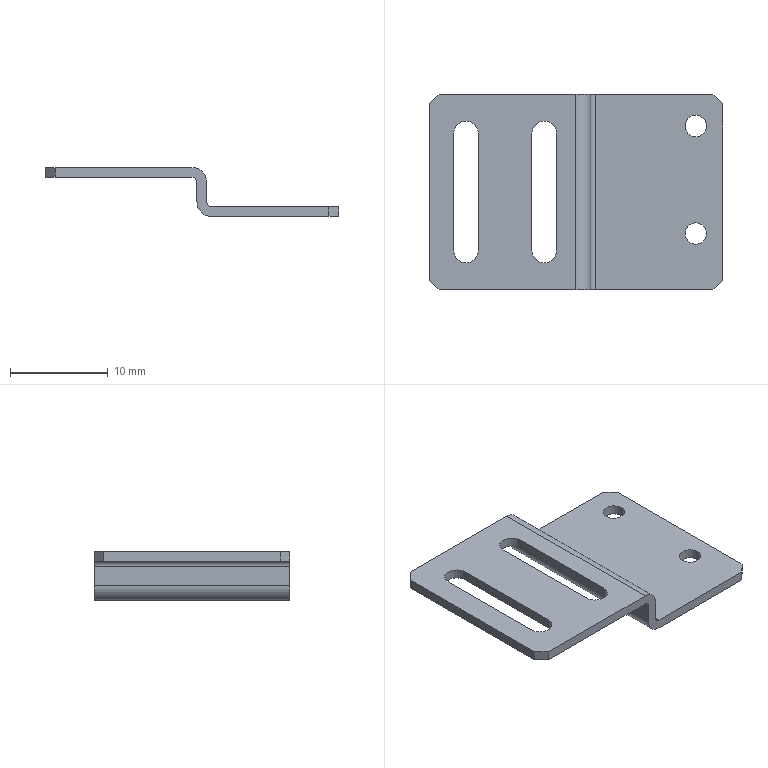Part | SolidWorks | features Fillet 2, Chamfer 1, Extrusion 1, HoleWzd 1, ICE 1 | 1 solid | 30 faces | box 30 x 20 x 5 mm | volume 583.412 mm3 | plane 18 | cylinder 12 | commonest cylinder face diameters 2.2 x4 2.5 x4 1 x2 3 x2
STEP:
#1=CARTESIAN_POINT('',(26.15,16.75,-5.));
#2=VERTEX_POINT('',#1);
#3=CARTESIAN_POINT('',(28.35,16.75,-5.));
#4=VERTEX_POINT('',#3);
#5=CARTESIAN_POINT('',(27.25,16.75,-5.));
#6=DIRECTION('',(0.,0.,1.));
#7=DIRECTION('',(1.,0.,0.));
#8=AXIS2_PLACEMENT_3D('',#5,#6,#7);
#9=CIRCLE('',#8,1.1);
#10=EDGE_CURVE('',#2,#4,#9,.T.);
#11=ORIENTED_EDGE('',*,*,#10,.F.);
#12=CARTESIAN_POINT('',(26.15,16.75,-4.));
#13=VERTEX_POINT('',#12);
#14=CARTESIAN_POINT('',(26.15,16.75,-4.));
#15=DIRECTION('',(0.,0.,1.));
#16=VECTOR('',#15,1000.);
#17=LINE('',#14,#16);
#18=EDGE_CURVE('',#2,#13,#17,.T.);
#19=ORIENTED_EDGE('',*,*,#18,.T.);
#20=CARTESIAN_POINT('',(28.35,16.75,-4.));
#21=VERTEX_POINT('',#20);
#22=CARTESIAN_POINT('',(27.25,16.75,-4.));
#23=DIRECTION('',(0.,0.,1.));
#24=DIRECTION('',(1.,0.,0.));
#25=AXIS2_PLACEMENT_3D('',#22,#23,#24);
#26=CIRCLE('',#25,1.1);
#27=EDGE_CURVE('',#13,#21,#26,.T.);
#28=ORIENTED_EDGE('',*,*,#27,.T.);
#29=CARTESIAN_POINT('',(28.35,16.75,-4.));
#30=DIRECTION('',(0.,0.,1.));
#31=VECTOR('',#30,1000.);
#32=LINE('',#29,#31);
#33=EDGE_CURVE('',#4,#21,#32,.T.);
#34=ORIENTED_EDGE('',*,*,#33,.F.);
#35=EDGE_LOOP('',(#11,#19,#28,#34));
#36=FACE_OUTER_BOUND('',#35,.T.);
#37=CARTESIAN_POINT('',(27.25,16.75,-4.));
#38=DIRECTION('',(0.,0.,1.));
#39=DIRECTION('',(1.,0.,0.));
#40=AXIS2_PLACEMENT_3D('',#37,#38,#39);
#41=CYLINDRICAL_SURFACE('',#40,1.1);
#42=ADVANCED_FACE('',(#36),#41,.F.);
#43=CARTESIAN_POINT('',(26.15,5.75,-5.));
#44=VERTEX_POINT('',#43);
#45=CARTESIAN_POINT('',(28.35,5.75,-5.));
#46=VERTEX_POINT('',#45);
#47=CARTESIAN_POINT('',(27.25,5.75,-5.));
#48=DIRECTION('',(0.,0.,1.));
#49=DIRECTION('',(1.,0.,0.));
#50=AXIS2_PLACEMENT_3D('',#47,#48,#49);
#51=CIRCLE('',#50,1.1);
#52=EDGE_CURVE('',#44,#46,#51,.T.);
#53=ORIENTED_EDGE('',*,*,#52,.F.);
#54=CARTESIAN_POINT('',(26.15,5.75,-4.));
#55=VERTEX_POINT('',#54);
#56=CARTESIAN_POINT('',(26.15,5.75,-4.));
#57=DIRECTION('',(0.,0.,1.));
#58=VECTOR('',#57,1000.);
#59=LINE('',#56,#58);
#60=EDGE_CURVE('',#44,#55,#59,.T.);
#61=ORIENTED_EDGE('',*,*,#60,.T.);
#62=CARTESIAN_POINT('',(28.35,5.75,-4.));
#63=VERTEX_POINT('',#62);
#64=CARTESIAN_POINT('',(27.25,5.75,-4.));
#65=DIRECTION('',(0.,0.,1.));
#66=DIRECTION('',(1.,0.,0.));
#67=AXIS2_PLACEMENT_3D('',#64,#65,#66);
#68=CIRCLE('',#67,1.1);
#69=EDGE_CURVE('',#55,#63,#68,.T.);
#70=ORIENTED_EDGE('',*,*,#69,.T.);
#71=CARTESIAN_POINT('',(28.35,5.75,-4.));
#72=DIRECTION('',(0.,0.,1.));
#73=VECTOR('',#72,1000.);
#74=LINE('',#71,#73);
#75=EDGE_CURVE('',#46,#63,#74,.T.);
#76=ORIENTED_EDGE('',*,*,#75,.F.);
#77=EDGE_LOOP('',(#53,#61,#70,#76));
#78=FACE_OUTER_BOUND('',#77,.T.);
#79=CARTESIAN_POINT('',(27.25,5.75,-4.));
#80=DIRECTION('',(0.,0.,1.));
#81=DIRECTION('',(1.,0.,0.));
#82=AXIS2_PLACEMENT_3D('',#79,#80,#81);
#83=CYLINDRICAL_SURFACE('',#82,1.1);
#84=ADVANCED_FACE('',(#78),#83,.F.);
#85=CARTESIAN_POINT('',(0.,19.,-1.));
#86=VERTEX_POINT('',#85);
#87=CARTESIAN_POINT('',(0.,1.,-1.));
#88=VERTEX_POINT('',#87);
#89=CARTESIAN_POINT('',(0.,20.,-1.));
#90=DIRECTION('',(0.,-1.,0.));
#91=VECTOR('',#90,1000.);
#92=LINE('',#89,#91);
#93=EDGE_CURVE('',#86,#88,#92,.T.);
#94=ORIENTED_EDGE('',*,*,#93,.T.);
#95=CARTESIAN_POINT('',(0.,1.,0.));
#96=VERTEX_POINT('',#95);
#97=CARTESIAN_POINT('',(0.,1.,0.));
#98=DIRECTION('',(0.,0.,1.));
#99=VECTOR('',#98,1000.);
#100=LINE('',#97,#99);
#101=EDGE_CURVE('',#88,#96,#100,.T.);
#102=ORIENTED_EDGE('',*,*,#101,.T.);
#103=CARTESIAN_POINT('',(0.,19.,0.));
#104=VERTEX_POINT('',#103);
#105=CARTESIAN_POINT('',(0.,20.,0.));
#106=DIRECTION('',(0.,-1.,0.));
#107=VECTOR('',#106,1000.);
#108=LINE('',#105,#107);
#109=EDGE_CURVE('',#104,#96,#108,.T.);
#110=ORIENTED_EDGE('',*,*,#109,.F.);
#111=CARTESIAN_POINT('',(0.,19.,0.));
#112=DIRECTION('',(0.,0.,-1.));
#113=VECTOR('',#112,1000.);
#114=LINE('',#111,#113);
#115=EDGE_CURVE('',#104,#86,#114,.T.);
#116=ORIENTED_EDGE('',*,*,#115,.T.);
#117=EDGE_LOOP('',(#94,#102,#110,#116));
#118=FACE_OUTER_BOUND('',#117,.T.);
#119=CARTESIAN_POINT('',(0.,20.,0.));
#120=DIRECTION('',(1.,0.,0.));
#121=DIRECTION('',(0.,0.,-1.));
#122=AXIS2_PLACEMENT_3D('',#119,#120,#121);
#123=PLANE('',#122);
#124=ADVANCED_FACE('',(#118),#123,.F.);
#125=CARTESIAN_POINT('',(2.5,4.,0.));
#126=VERTEX_POINT('',#125);
#127=CARTESIAN_POINT('',(2.5,16.,0.));
#128=VERTEX_POINT('',#127);
#129=CARTESIAN_POINT('',(2.5,20.,0.));
#130=DIRECTION('',(0.,1.,0.));
#131=VECTOR('',#130,1000.);
#132=LINE('',#129,#131);
#133=EDGE_CURVE('',#126,#128,#132,.T.);
#134=ORIENTED_EDGE('',*,*,#133,.T.);
#135=CARTESIAN_POINT('',(5.,16.,0.));
#136=VERTEX_POINT('',#135);
#137=CARTESIAN_POINT('',(3.75,16.,0.));
#138=DIRECTION('',(0.,0.,-1.));
#139=DIRECTION('',(-1.,0.,0.));
#140=AXIS2_PLACEMENT_3D('',#137,#138,#139);
#141=CIRCLE('',#140,1.25);
#142=EDGE_CURVE('',#128,#136,#141,.T.);
#143=ORIENTED_EDGE('',*,*,#142,.T.);
#144=CARTESIAN_POINT('',(5.,4.,0.));
#145=VERTEX_POINT('',#144);
#146=CARTESIAN_POINT('',(5.,20.,0.));
#147=DIRECTION('',(0.,-1.,0.));
#148=VECTOR('',#147,1000.);
#149=LINE('',#146,#148);
#150=EDGE_CURVE('',#136,#145,#149,.T.);
#151=ORIENTED_EDGE('',*,*,#150,.T.);
#152=CARTESIAN_POINT('',(3.75,4.,0.));
#153=DIRECTION('',(0.,0.,-1.));
#154=DIRECTION('',(-1.,0.,0.));
#155=AXIS2_PLACEMENT_3D('',#152,#153,#154);
#156=CIRCLE('',#155,1.25);
#157=EDGE_CURVE('',#145,#126,#156,.T.);
#158=ORIENTED_EDGE('',*,*,#157,.T.);
#159=EDGE_LOOP('',(#134,#143,#151,#158));
#160=FACE_BOUND('',#159,.T.);
#161=CARTESIAN_POINT('',(10.5,4.,0.));
#162=VERTEX_POINT('',#161);
#163=CARTESIAN_POINT('',(10.5,16.,0.));
#164=VERTEX_POINT('',#163);
#165=CARTESIAN_POINT('',(10.5,20.,0.));
#166=DIRECTION('',(0.,1.,0.));
#167=VECTOR('',#166,1000.);
#168=LINE('',#165,#167);
#169=EDGE_CURVE('',#162,#164,#168,.T.);
#170=ORIENTED_EDGE('',*,*,#169,.T.);
#171=CARTESIAN_POINT('',(13.,16.,0.));
#172=VERTEX_POINT('',#171);
#173=CARTESIAN_POINT('',(11.75,16.,0.));
#174=DIRECTION('',(0.,0.,-1.));
#175=DIRECTION('',(-1.,0.,0.));
#176=AXIS2_PLACEMENT_3D('',#173,#174,#175);
#177=CIRCLE('',#176,1.25);
#178=EDGE_CURVE('',#164,#172,#177,.T.);
#179=ORIENTED_EDGE('',*,*,#178,.T.);
#180=CARTESIAN_POINT('',(13.,4.,0.));
#181=VERTEX_POINT('',#180);
#182=CARTESIAN_POINT('',(13.,20.,0.));
#183=DIRECTION('',(0.,-1.,0.));
#184=VECTOR('',#183,1000.);
#185=LINE('',#182,#184);
#186=EDGE_CURVE('',#172,#181,#185,.T.);
#187=ORIENTED_EDGE('',*,*,#186,.T.);
#188=CARTESIAN_POINT('',(11.75,4.,0.));
#189=DIRECTION('',(0.,0.,-1.));
#190=DIRECTION('',(-1.,0.,0.));
#191=AXIS2_PLACEMENT_3D('',#188,#189,#190);
#192=CIRCLE('',#191,1.25);
#193=EDGE_CURVE('',#181,#162,#192,.T.);
#194=ORIENTED_EDGE('',*,*,#193,.T.);
#195=EDGE_LOOP('',(#170,#179,#187,#194));
#196=FACE_BOUND('',#195,.T.);
#197=CARTESIAN_POINT('',(1.,0.,0.));
#198=VERTEX_POINT('',#197);
#199=CARTESIAN_POINT('',(15.,0.,0.));
#200=VERTEX_POINT('',#199);
#201=CARTESIAN_POINT('',(0.,0.,0.));
#202=DIRECTION('',(1.,0.,0.));
#203=VECTOR('',#202,1000.);
#204=LINE('',#201,#203);
#205=EDGE_CURVE('',#198,#200,#204,.T.);
#206=ORIENTED_EDGE('',*,*,#205,.T.);
#207=CARTESIAN_POINT('',(15.,20.,0.));
#208=VERTEX_POINT('',#207);
#209=CARTESIAN_POINT('',(15.,20.,0.));
#210=DIRECTION('',(0.,1.,0.));
#211=VECTOR('',#210,1000.);
#212=LINE('',#209,#211);
#213=EDGE_CURVE('',#200,#208,#212,.T.);
#214=ORIENTED_EDGE('',*,*,#213,.T.);
#215=CARTESIAN_POINT('',(1.,20.,0.));
#216=VERTEX_POINT('',#215);
#217=CARTESIAN_POINT('',(0.,20.,0.));
#218=DIRECTION('',(1.,0.,0.));
#219=VECTOR('',#218,1000.);
#220=LINE('',#217,#219);
#221=EDGE_CURVE('',#216,#208,#220,.T.);
#222=ORIENTED_EDGE('',*,*,#221,.F.);
#223=CARTESIAN_POINT('',(1.,20.,0.));
#224=DIRECTION('',(-0.7071,-0.7071,0.));
#225=VECTOR('',#224,1000.);
#226=LINE('',#223,#225);
#227=EDGE_CURVE('',#216,#104,#226,.T.);
#228=ORIENTED_EDGE('',*,*,#227,.T.);
#229=ORIENTED_EDGE('',*,*,#109,.T.);
#230=CARTESIAN_POINT('',(0.,1.,0.));
#231=DIRECTION('',(0.7071,-0.7071,0.));
#232=VECTOR('',#231,1000.);
#233=LINE('',#230,#232);
#234=EDGE_CURVE('',#96,#198,#233,.T.);
#235=ORIENTED_EDGE('',*,*,#234,.T.);
#236=EDGE_LOOP('',(#206,#214,#222,#228,#229,#235));
#237=FACE_OUTER_BOUND('',#236,.T.);
#238=CARTESIAN_POINT('',(0.,20.,0.));
#239=DIRECTION('',(0.,0.,-1.));
#240=DIRECTION('',(-1.,0.,0.));
#241=AXIS2_PLACEMENT_3D('',#238,#239,#240);
#242=PLANE('',#241);
#243=ADVANCED_FACE('',(#160,#196,#237),#242,.F.);
#244=CARTESIAN_POINT('',(16.5,0.,-1.5));
#245=VERTEX_POINT('',#244);
#246=CARTESIAN_POINT('',(16.5,0.,-3.5));
#247=VERTEX_POINT('',#246);
#248=CARTESIAN_POINT('',(16.5,0.,0.));
#249=DIRECTION('',(0.,0.,-1.));
#250=VECTOR('',#249,1000.);
#251=LINE('',#248,#250);
#252=EDGE_CURVE('',#245,#247,#251,.T.);
#253=ORIENTED_EDGE('',*,*,#252,.T.);
#254=CARTESIAN_POINT('',(16.5,20.,-3.5));
#255=VERTEX_POINT('',#254);
#256=CARTESIAN_POINT('',(16.5,20.,-3.5));
#257=DIRECTION('',(0.,1.,0.));
#258=VECTOR('',#257,1000.);
#259=LINE('',#256,#258);
#260=EDGE_CURVE('',#247,#255,#259,.T.);
#261=ORIENTED_EDGE('',*,*,#260,.T.);
#262=CARTESIAN_POINT('',(16.5,20.,-1.5));
#263=VERTEX_POINT('',#262);
#264=CARTESIAN_POINT('',(16.5,20.,0.));
#265=DIRECTION('',(0.,0.,-1.));
#266=VECTOR('',#265,1000.);
#267=LINE('',#264,#266);
#268=EDGE_CURVE('',#263,#255,#267,.T.);
#269=ORIENTED_EDGE('',*,*,#268,.F.);
#270=CARTESIAN_POINT('',(16.5,20.,-1.5));
#271=DIRECTION('',(0.,-1.,0.));
#272=VECTOR('',#271,1000.);
#273=LINE('',#270,#272);
#274=EDGE_CURVE('',#263,#245,#273,.T.);
#275=ORIENTED_EDGE('',*,*,#274,.T.);
#276=EDGE_LOOP('',(#253,#261,#269,#275));
#277=FACE_OUTER_BOUND('',#276,.T.);
#278=CARTESIAN_POINT('',(16.5,20.,0.));
#279=DIRECTION('',(-1.,0.,0.));
#280=DIRECTION('',(0.,0.,1.));
#281=AXIS2_PLACEMENT_3D('',#278,#279,#280);
#282=PLANE('',#281);
#283=ADVANCED_FACE('',(#277),#282,.F.);
#284=CARTESIAN_POINT('',(27.25,16.75,-4.));
#285=DIRECTION('',(0.,0.,1.));
#286=DIRECTION('',(1.,0.,0.));
#287=AXIS2_PLACEMENT_3D('',#284,#285,#286);
#288=CIRCLE('',#287,1.1);
#289=EDGE_CURVE('',#21,#13,#288,.T.);
#290=ORIENTED_EDGE('',*,*,#289,.F.);
#291=ORIENTED_EDGE('',*,*,#27,.F.);
#292=EDGE_LOOP('',(#290,#291));
#293=FACE_BOUND('',#292,.T.);
#294=CARTESIAN_POINT('',(27.25,5.75,-4.));
#295=DIRECTION('',(0.,0.,1.));
#296=DIRECTION('',(1.,0.,0.));
#297=AXIS2_PLACEMENT_3D('',#294,#295,#296);
#298=CIRCLE('',#297,1.1);
#299=EDGE_CURVE('',#63,#55,#298,.T.);
#300=ORIENTED_EDGE('',*,*,#299,.F.);
#301=ORIENTED_EDGE('',*,*,#69,.F.);
#302=EDGE_LOOP('',(#300,#301));
#303=FACE_BOUND('',#302,.T.);
#304=CARTESIAN_POINT('',(17.,20.,-4.));
#305=VERTEX_POINT('',#304);
#306=CARTESIAN_POINT('',(29.,20.,-4.));
#307=VERTEX_POINT('',#306);
#308=CARTESIAN_POINT('',(30.,20.,-4.));
#309=DIRECTION('',(1.,0.,0.));
#310=VECTOR('',#309,1000.);
#311=LINE('',#308,#310);
#312=EDGE_CURVE('',#305,#307,#311,.T.);
#313=ORIENTED_EDGE('',*,*,#312,.F.);
#314=CARTESIAN_POINT('',(17.,0.,-4.));
#315=VERTEX_POINT('',#314);
#316=CARTESIAN_POINT('',(17.,0.,-4.));
#317=DIRECTION('',(0.,-1.,0.));
#318=VECTOR('',#317,1000.);
#319=LINE('',#316,#318);
#320=EDGE_CURVE('',#305,#315,#319,.T.);
#321=ORIENTED_EDGE('',*,*,#320,.T.);
#322=CARTESIAN_POINT('',(29.,0.,-4.));
#323=VERTEX_POINT('',#322);
#324=CARTESIAN_POINT('',(30.,0.,-4.));
#325=DIRECTION('',(1.,0.,0.));
#326=VECTOR('',#325,1000.);
#327=LINE('',#324,#326);
#328=EDGE_CURVE('',#315,#323,#327,.T.);
#329=ORIENTED_EDGE('',*,*,#328,.T.);
#330=CARTESIAN_POINT('',(30.,1.,-4.));
#331=VERTEX_POINT('',#330);
#332=CARTESIAN_POINT('',(30.,1.,-4.));
#333=DIRECTION('',(0.7071,0.7071,0.));
#334=VECTOR('',#333,1000.);
#335=LINE('',#332,#334);
#336=EDGE_CURVE('',#323,#331,#335,.T.);
#337=ORIENTED_EDGE('',*,*,#336,.T.);
#338=CARTESIAN_POINT('',(30.,19.,-4.));
#339=VERTEX_POINT('',#338);
#340=CARTESIAN_POINT('',(30.,20.,-4.));
#341=DIRECTION('',(0.,-1.,0.));
#342=VECTOR('',#341,1000.);
#343=LINE('',#340,#342);
#344=EDGE_CURVE('',#339,#331,#343,.T.);
#345=ORIENTED_EDGE('',*,*,#344,.F.);
#346=CARTESIAN_POINT('',(29.,20.,-4.));
#347=DIRECTION('',(-0.7071,0.7071,0.));
#348=VECTOR('',#347,1000.);
#349=LINE('',#346,#348);
#350=EDGE_CURVE('',#339,#307,#349,.T.);
#351=ORIENTED_EDGE('',*,*,#350,.T.);
#352=EDGE_LOOP('',(#313,#321,#329,#337,#345,#351));
#353=FACE_OUTER_BOUND('',#352,.T.);
#354=CARTESIAN_POINT('',(30.,20.,-4.));
#355=DIRECTION('',(0.,0.,-1.));
#356=DIRECTION('',(-1.,0.,0.));
#357=AXIS2_PLACEMENT_3D('',#354,#355,#356);
#358=PLANE('',#357);
#359=ADVANCED_FACE('',(#293,#303,#353),#358,.F.);
#360=ORIENTED_EDGE('',*,*,#344,.T.);
#361=CARTESIAN_POINT('',(30.,1.,-5.));
#362=VERTEX_POINT('',#361);
#363=CARTESIAN_POINT('',(30.,1.,-5.));
#364=DIRECTION('',(0.,0.,-1.));
#365=VECTOR('',#364,1000.);
#366=LINE('',#363,#365);
#367=EDGE_CURVE('',#331,#362,#366,.T.);
#368=ORIENTED_EDGE('',*,*,#367,.T.);
#369=CARTESIAN_POINT('',(30.,19.,-5.));
#370=VERTEX_POINT('',#369);
#371=CARTESIAN_POINT('',(30.,20.,-5.));
#372=DIRECTION('',(0.,-1.,0.));
#373=VECTOR('',#372,1000.);
#374=LINE('',#371,#373);
#375=EDGE_CURVE('',#370,#362,#374,.T.);
#376=ORIENTED_EDGE('',*,*,#375,.F.);
#377=CARTESIAN_POINT('',(30.,19.,-4.));
#378=DIRECTION('',(0.,0.,1.));
#379=VECTOR('',#378,1000.);
#380=LINE('',#377,#379);
#381=EDGE_CURVE('',#370,#339,#380,.T.);
#382=ORIENTED_EDGE('',*,*,#381,.T.);
#383=EDGE_LOOP('',(#360,#368,#376,#382));
#384=FACE_OUTER_BOUND('',#383,.T.);
#385=CARTESIAN_POINT('',(30.,20.,-4.));
#386=DIRECTION('',(-1.,0.,0.));
#387=DIRECTION('',(0.,0.,1.));
#388=AXIS2_PLACEMENT_3D('',#385,#386,#387);
#389=PLANE('',#388);
#390=ADVANCED_FACE('',(#384),#389,.F.);
#391=CARTESIAN_POINT('',(27.25,16.75,-5.));
#392=DIRECTION('',(0.,0.,1.));
#393=DIRECTION('',(1.,0.,0.));
#394=AXIS2_PLACEMENT_3D('',#391,#392,#393);
#395=CIRCLE('',#394,1.1);
#396=EDGE_CURVE('',#4,#2,#395,.T.);
#397=ORIENTED_EDGE('',*,*,#396,.T.);
#398=ORIENTED_EDGE('',*,*,#10,.T.);
#399=EDGE_LOOP('',(#397,#398));
#400=FACE_BOUND('',#399,.T.);
#401=CARTESIAN_POINT('',(27.25,5.75,-5.));
#402=DIRECTION('',(0.,0.,1.));
#403=DIRECTION('',(1.,0.,0.));
#404=AXIS2_PLACEMENT_3D('',#401,#402,#403);
#405=CIRCLE('',#404,1.1);
#406=EDGE_CURVE('',#46,#44,#405,.T.);
#407=ORIENTED_EDGE('',*,*,#406,.T.);
#408=ORIENTED_EDGE('',*,*,#52,.T.);
#409=EDGE_LOOP('',(#407,#408));
#410=FACE_BOUND('',#409,.T.);
#411=CARTESIAN_POINT('',(29.,0.,-5.));
#412=VERTEX_POINT('',#411);
#413=CARTESIAN_POINT('',(17.,0.,-5.));
#414=VERTEX_POINT('',#413);
#415=CARTESIAN_POINT('',(15.5,0.,-5.));
#416=DIRECTION('',(-1.,0.,0.));
#417=VECTOR('',#416,1000.);
#418=LINE('',#415,#417);
#419=EDGE_CURVE('',#412,#414,#418,.T.);
#420=ORIENTED_EDGE('',*,*,#419,.T.);
#421=CARTESIAN_POINT('',(17.,20.,-5.));
#422=VERTEX_POINT('',#421);
#423=CARTESIAN_POINT('',(17.,20.,-5.));
#424=DIRECTION('',(0.,1.,0.));
#425=VECTOR('',#424,1000.);
#426=LINE('',#423,#425);
#427=EDGE_CURVE('',#414,#422,#426,.T.);
#428=ORIENTED_EDGE('',*,*,#427,.T.);
#429=CARTESIAN_POINT('',(29.,20.,-5.));
#430=VERTEX_POINT('',#429);
#431=CARTESIAN_POINT('',(15.5,20.,-5.));
#432=DIRECTION('',(-1.,0.,0.));
#433=VECTOR('',#432,1000.);
#434=LINE('',#431,#433);
#435=EDGE_CURVE('',#430,#422,#434,.T.);
#436=ORIENTED_EDGE('',*,*,#435,.F.);
#437=CARTESIAN_POINT('',(29.,20.,-5.));
#438=DIRECTION('',(0.7071,-0.7071,0.));
#439=VECTOR('',#438,1000.);
#440=LINE('',#437,#439);
#441=EDGE_CURVE('',#430,#370,#440,.T.);
#442=ORIENTED_EDGE('',*,*,#441,.T.);
#443=ORIENTED_EDGE('',*,*,#375,.T.);
#444=CARTESIAN_POINT('',(30.,1.,-5.));
#445=DIRECTION('',(-0.7071,-0.7071,0.));
#446=VECTOR('',#445,1000.);
#447=LINE('',#444,#446);
#448=EDGE_CURVE('',#362,#412,#447,.T.);
#449=ORIENTED_EDGE('',*,*,#448,.T.);
#450=EDGE_LOOP('',(#420,#428,#436,#442,#443,#449));
#451=FACE_OUTER_BOUND('',#450,.T.);
#452=CARTESIAN_POINT('',(15.5,20.,-5.));
#453=DIRECTION('',(0.,0.,1.));
#454=DIRECTION('',(1.,0.,0.));
#455=AXIS2_PLACEMENT_3D('',#452,#453,#454);
#456=PLANE('',#455);
#457=ADVANCED_FACE('',(#400,#410,#451),#456,.F.);
#458=CARTESIAN_POINT('',(15.5,0.,-3.5));
#459=VERTEX_POINT('',#458);
#460=CARTESIAN_POINT('',(15.5,0.,-1.5));
#461=VERTEX_POINT('',#460);
#462=CARTESIAN_POINT('',(15.5,0.,-5.));
#463=DIRECTION('',(0.,0.,1.));
#464=VECTOR('',#463,1000.);
#465=LINE('',#462,#464);
#466=EDGE_CURVE('',#459,#461,#465,.T.);
#467=ORIENTED_EDGE('',*,*,#466,.T.);
#468=CARTESIAN_POINT('',(15.5,20.,-1.5));
#469=VERTEX_POINT('',#468);
#470=CARTESIAN_POINT('',(15.5,20.,-1.5));
#471=DIRECTION('',(0.,1.,0.));
#472=VECTOR('',#471,1000.);
#473=LINE('',#470,#472);
#474=EDGE_CURVE('',#461,#469,#473,.T.);
#475=ORIENTED_EDGE('',*,*,#474,.T.);
#476=CARTESIAN_POINT('',(15.5,20.,-3.5));
#477=VERTEX_POINT('',#476);
#478=CARTESIAN_POINT('',(15.5,20.,-5.));
#479=DIRECTION('',(0.,0.,1.));
#480=VECTOR('',#479,1000.);
#481=LINE('',#478,#480);
#482=EDGE_CURVE('',#477,#469,#481,.T.);
#483=ORIENTED_EDGE('',*,*,#482,.F.);
#484=CARTESIAN_POINT('',(15.5,20.,-3.5));
#485=DIRECTION('',(0.,-1.,0.));
#486=VECTOR('',#485,1000.);
#487=LINE('',#484,#486);
#488=EDGE_CURVE('',#477,#459,#487,.T.);
#489=ORIENTED_EDGE('',*,*,#488,.T.);
#490=EDGE_LOOP('',(#467,#475,#483,#489));
#491=FACE_OUTER_BOUND('',#490,.T.);
#492=CARTESIAN_POINT('',(15.5,20.,-5.));
#493=DIRECTION('',(1.,0.,0.));
#494=DIRECTION('',(0.,0.,-1.));
#495=AXIS2_PLACEMENT_3D('',#492,#493,#494);
#496=PLANE('',#495);
#497=ADVANCED_FACE('',(#491),#496,.F.);
#498=CARTESIAN_POINT('',(5.,4.,-1.));
#499=VERTEX_POINT('',#498);
#500=CARTESIAN_POINT('',(5.,16.,-1.));
#501=VERTEX_POINT('',#500);
#502=CARTESIAN_POINT('',(5.,20.,-1.));
#503=DIRECTION('',(0.,1.,0.));
#504=VECTOR('',#503,1000.);
#505=LINE('',#502,#504);
#506=EDGE_CURVE('',#499,#501,#505,.T.);
#507=ORIENTED_EDGE('',*,*,#506,.T.);
#508=CARTESIAN_POINT('',(2.5,16.,-1.));
#509=VERTEX_POINT('',#508);
#510=CARTESIAN_POINT('',(3.75,16.,-1.));
#511=DIRECTION('',(0.,0.,1.));
#512=DIRECTION('',(1.,0.,0.));
#513=AXIS2_PLACEMENT_3D('',#510,#511,#512);
#514=CIRCLE('',#513,1.25);
#515=EDGE_CURVE('',#501,#509,#514,.T.);
#516=ORIENTED_EDGE('',*,*,#515,.T.);
#517=CARTESIAN_POINT('',(2.5,4.,-1.));
#518=VERTEX_POINT('',#517);
#519=CARTESIAN_POINT('',(2.5,20.,-1.));
#520=DIRECTION('',(0.,-1.,0.));
#521=VECTOR('',#520,1000.);
#522=LINE('',#519,#521);
#523=EDGE_CURVE('',#509,#518,#522,.T.);
#524=ORIENTED_EDGE('',*,*,#523,.T.);
#525=CARTESIAN_POINT('',(3.75,4.,-1.));
#526=DIRECTION('',(0.,0.,1.));
#527=DIRECTION('',(1.,0.,0.));
#528=AXIS2_PLACEMENT_3D('',#525,#526,#527);
#529=CIRCLE('',#528,1.25);
#530=EDGE_CURVE('',#518,#499,#529,.T.);
#531=ORIENTED_EDGE('',*,*,#530,.T.);
#532=EDGE_LOOP('',(#507,#516,#524,#531));
#533=FACE_BOUND('',#532,.T.);
#534=CARTESIAN_POINT('',(13.,4.,-1.));
#535=VERTEX_POINT('',#534);
#536=CARTESIAN_POINT('',(13.,16.,-1.));
#537=VERTEX_POINT('',#536);
#538=CARTESIAN_POINT('',(13.,20.,-1.));
#539=DIRECTION('',(0.,1.,0.));
#540=VECTOR('',#539,1000.);
#541=LINE('',#538,#540);
#542=EDGE_CURVE('',#535,#537,#541,.T.);
#543=ORIENTED_EDGE('',*,*,#542,.T.);
#544=CARTESIAN_POINT('',(10.5,16.,-1.));
#545=VERTEX_POINT('',#544);
#546=CARTESIAN_POINT('',(11.75,16.,-1.));
#547=DIRECTION('',(0.,0.,1.));
#548=DIRECTION('',(1.,0.,0.));
#549=AXIS2_PLACEMENT_3D('',#546,#547,#548);
#550=CIRCLE('',#549,1.25);
#551=EDGE_CURVE('',#537,#545,#550,.T.);
#552=ORIENTED_EDGE('',*,*,#551,.T.);
#553=CARTESIAN_POINT('',(10.5,4.,-1.));
#554=VERTEX_POINT('',#553);
#555=CARTESIAN_POINT('',(10.5,20.,-1.));
#556=DIRECTION('',(0.,-1.,0.));
#557=VECTOR('',#556,1000.);
#558=LINE('',#555,#557);
#559=EDGE_CURVE('',#545,#554,#558,.T.);
#560=ORIENTED_EDGE('',*,*,#559,.T.);
#561=CARTESIAN_POINT('',(11.75,4.,-1.));
#562=DIRECTION('',(0.,0.,1.));
#563=DIRECTION('',(1.,0.,0.));
#564=AXIS2_PLACEMENT_3D('',#561,#562,#563);
#565=CIRCLE('',#564,1.25);
#566=EDGE_CURVE('',#554,#535,#565,.T.);
#567=ORIENTED_EDGE('',*,*,#566,.T.);
#568=EDGE_LOOP('',(#543,#552,#560,#567));
#569=FACE_BOUND('',#568,.T.);
#570=CARTESIAN_POINT('',(15.,20.,-1.));
#571=VERTEX_POINT('',#570);
#572=CARTESIAN_POINT('',(1.,20.,-1.));
#573=VERTEX_POINT('',#572);
#574=CARTESIAN_POINT('',(0.,20.,-1.));
#575=DIRECTION('',(-1.,0.,0.));
#576=VECTOR('',#575,1000.);
#577=LINE('',#574,#576);
#578=EDGE_CURVE('',#571,#573,#577,.T.);
#579=ORIENTED_EDGE('',*,*,#578,.F.);
#580=CARTESIAN_POINT('',(15.,0.,-1.));
#581=VERTEX_POINT('',#580);
#582=CARTESIAN_POINT('',(15.,0.,-1.));
#583=DIRECTION('',(0.,-1.,0.));
#584=VECTOR('',#583,1000.);
#585=LINE('',#582,#584);
#586=EDGE_CURVE('',#571,#581,#585,.T.);
#587=ORIENTED_EDGE('',*,*,#586,.T.);
#588=CARTESIAN_POINT('',(1.,0.,-1.));
#589=VERTEX_POINT('',#588);
#590=CARTESIAN_POINT('',(0.,0.,-1.));
#591=DIRECTION('',(-1.,0.,0.));
#592=VECTOR('',#591,1000.);
#593=LINE('',#590,#592);
#594=EDGE_CURVE('',#581,#589,#593,.T.);
#595=ORIENTED_EDGE('',*,*,#594,.T.);
#596=CARTESIAN_POINT('',(0.,1.,-1.));
#597=DIRECTION('',(-0.7071,0.7071,0.));
#598=VECTOR('',#597,1000.);
#599=LINE('',#596,#598);
#600=EDGE_CURVE('',#589,#88,#599,.T.);
#601=ORIENTED_EDGE('',*,*,#600,.T.);
#602=ORIENTED_EDGE('',*,*,#93,.F.);
#603=CARTESIAN_POINT('',(1.,20.,-1.));
#604=DIRECTION('',(0.7071,0.7071,0.));
#605=VECTOR('',#604,1000.);
#606=LINE('',#603,#605);
#607=EDGE_CURVE('',#86,#573,#606,.T.);
#608=ORIENTED_EDGE('',*,*,#607,.T.);
#609=EDGE_LOOP('',(#579,#587,#595,#601,#602,#608));
#610=FACE_OUTER_BOUND('',#609,.T.);
#611=CARTESIAN_POINT('',(0.,20.,-1.));
#612=DIRECTION('',(0.,0.,1.));
#613=DIRECTION('',(1.,0.,0.));
#614=AXIS2_PLACEMENT_3D('',#611,#612,#613);
#615=PLANE('',#614);
#616=ADVANCED_FACE('',(#533,#569,#610),#615,.F.);
#617=ORIENTED_EDGE('',*,*,#221,.T.);
#618=CARTESIAN_POINT('',(15.,20.,-1.5));
#619=DIRECTION('',(0.,1.,0.));
#620=DIRECTION('',(0.,0.,-1.));
#621=AXIS2_PLACEMENT_3D('',#618,#619,#620);
#622=CIRCLE('',#621,1.5);
#623=EDGE_CURVE('',#208,#263,#622,.T.);
#624=ORIENTED_EDGE('',*,*,#623,.T.);
#625=ORIENTED_EDGE('',*,*,#268,.T.);
#626=CARTESIAN_POINT('',(17.,20.,-3.5));
#627=DIRECTION('',(0.,-1.,0.));
#628=DIRECTION('',(0.,0.,-1.));
#629=AXIS2_PLACEMENT_3D('',#626,#627,#628);
#630=CIRCLE('',#629,0.5);
#631=EDGE_CURVE('',#255,#305,#630,.T.);
#632=ORIENTED_EDGE('',*,*,#631,.T.);
#633=ORIENTED_EDGE('',*,*,#312,.T.);
#634=CARTESIAN_POINT('',(29.,20.,0.));
#635=DIRECTION('',(0.,0.,-1.));
#636=VECTOR('',#635,1000.);
#637=LINE('',#634,#636);
#638=EDGE_CURVE('',#307,#430,#637,.T.);
#639=ORIENTED_EDGE('',*,*,#638,.T.);
#640=ORIENTED_EDGE('',*,*,#435,.T.);
#641=CARTESIAN_POINT('',(17.,20.,-3.5));
#642=DIRECTION('',(0.,1.,0.));
#643=DIRECTION('',(0.,0.,-1.));
#644=AXIS2_PLACEMENT_3D('',#641,#642,#643);
#645=CIRCLE('',#644,1.5);
#646=EDGE_CURVE('',#422,#477,#645,.T.);
#647=ORIENTED_EDGE('',*,*,#646,.T.);
#648=ORIENTED_EDGE('',*,*,#482,.T.);
#649=CARTESIAN_POINT('',(15.,20.,-1.5));
#650=DIRECTION('',(0.,-1.,0.));
#651=DIRECTION('',(0.,0.,-1.));
#652=AXIS2_PLACEMENT_3D('',#649,#650,#651);
#653=CIRCLE('',#652,0.5);
#654=EDGE_CURVE('',#469,#571,#653,.T.);
#655=ORIENTED_EDGE('',*,*,#654,.T.);
#656=ORIENTED_EDGE('',*,*,#578,.T.);
#657=CARTESIAN_POINT('',(1.,20.,0.));
#658=DIRECTION('',(0.,0.,1.));
#659=VECTOR('',#658,1000.);
#660=LINE('',#657,#659);
#661=EDGE_CURVE('',#573,#216,#660,.T.);
#662=ORIENTED_EDGE('',*,*,#661,.T.);
#663=EDGE_LOOP('',(#617,#624,#625,#632,#633,#639,#640,#647,#648,#655,#656,#662));
#664=FACE_OUTER_BOUND('',#663,.T.);
#665=CARTESIAN_POINT('',(0.,20.,0.));
#666=DIRECTION('',(0.,-1.,0.));
#667=DIRECTION('',(0.,0.,-1.));
#668=AXIS2_PLACEMENT_3D('',#665,#666,#667);
#669=PLANE('',#668);
#670=ADVANCED_FACE('',(#664),#669,.F.);
#671=ORIENTED_EDGE('',*,*,#252,.F.);
#672=CARTESIAN_POINT('',(15.,0.,-1.5));
#673=DIRECTION('',(0.,-1.,0.));
#674=DIRECTION('',(0.,0.,-1.));
#675=AXIS2_PLACEMENT_3D('',#672,#673,#674);
#676=CIRCLE('',#675,1.5);
#677=EDGE_CURVE('',#245,#200,#676,.T.);
#678=ORIENTED_EDGE('',*,*,#677,.T.);
#679=ORIENTED_EDGE('',*,*,#205,.F.);
#680=CARTESIAN_POINT('',(1.,0.,-1.));
#681=DIRECTION('',(0.,0.,-1.));
#682=VECTOR('',#681,1000.);
#683=LINE('',#680,#682);
#684=EDGE_CURVE('',#198,#589,#683,.T.);
#685=ORIENTED_EDGE('',*,*,#684,.T.);
#686=ORIENTED_EDGE('',*,*,#594,.F.);
#687=CARTESIAN_POINT('',(15.,0.,-1.5));
#688=DIRECTION('',(0.,1.,0.));
#689=DIRECTION('',(0.,0.,-1.));
#690=AXIS2_PLACEMENT_3D('',#687,#688,#689);
#691=CIRCLE('',#690,0.5);
#692=EDGE_CURVE('',#581,#461,#691,.T.);
#693=ORIENTED_EDGE('',*,*,#692,.T.);
#694=ORIENTED_EDGE('',*,*,#466,.F.);
#695=CARTESIAN_POINT('',(17.,0.,-3.5));
#696=DIRECTION('',(0.,-1.,0.));
#697=DIRECTION('',(0.,0.,-1.));
#698=AXIS2_PLACEMENT_3D('',#695,#696,#697);
#699=CIRCLE('',#698,1.5);
#700=EDGE_CURVE('',#459,#414,#699,.T.);
#701=ORIENTED_EDGE('',*,*,#700,.T.);
#702=ORIENTED_EDGE('',*,*,#419,.F.);
#703=CARTESIAN_POINT('',(29.,0.,-4.));
#704=DIRECTION('',(0.,0.,1.));
#705=VECTOR('',#704,1000.);
#706=LINE('',#703,#705);
#707=EDGE_CURVE('',#412,#323,#706,.T.);
#708=ORIENTED_EDGE('',*,*,#707,.T.);
#709=ORIENTED_EDGE('',*,*,#328,.F.);
#710=CARTESIAN_POINT('',(17.,0.,-3.5));
#711=DIRECTION('',(0.,1.,0.));
#712=DIRECTION('',(0.,0.,-1.));
#713=AXIS2_PLACEMENT_3D('',#710,#711,#712);
#714=CIRCLE('',#713,0.5);
#715=EDGE_CURVE('',#315,#247,#714,.T.);
#716=ORIENTED_EDGE('',*,*,#715,.T.);
#717=EDGE_LOOP('',(#671,#678,#679,#685,#686,#693,#694,#701,#702,#708,#709,#716));
#718=FACE_OUTER_BOUND('',#717,.T.);
#719=CARTESIAN_POINT('',(0.,0.,0.));
#720=DIRECTION('',(0.,-1.,0.));
#721=DIRECTION('',(0.,0.,-1.));
#722=AXIS2_PLACEMENT_3D('',#719,#720,#721);
#723=PLANE('',#722);
#724=ADVANCED_FACE('',(#718),#723,.T.);
#725=CARTESIAN_POINT('',(10.5,16.,5.));
#726=DIRECTION('',(0.,0.,-1.));
#727=VECTOR('',#726,1000.);
#728=LINE('',#725,#727);
#729=EDGE_CURVE('',#164,#545,#728,.T.);
#730=ORIENTED_EDGE('',*,*,#729,.T.);
#731=ORIENTED_EDGE('',*,*,#551,.F.);
#732=CARTESIAN_POINT('',(13.,16.,5.));
#733=DIRECTION('',(0.,0.,-1.));
#734=VECTOR('',#733,1000.);
#735=LINE('',#732,#734);
#736=EDGE_CURVE('',#172,#537,#735,.T.);
#737=ORIENTED_EDGE('',*,*,#736,.F.);
#738=ORIENTED_EDGE('',*,*,#178,.F.);
#739=EDGE_LOOP('',(#730,#731,#737,#738));
#740=FACE_OUTER_BOUND('',#739,.T.);
#741=CARTESIAN_POINT('',(11.75,16.,5.));
#742=DIRECTION('',(0.,0.,-1.));
#743=DIRECTION('',(-1.,0.,0.));
#744=AXIS2_PLACEMENT_3D('',#741,#742,#743);
#745=CYLINDRICAL_SURFACE('',#744,1.25);
#746=ADVANCED_FACE('',(#740),#745,.F.);
#747=CARTESIAN_POINT('',(10.5,4.,5.));
#748=DIRECTION('',(0.,0.,-1.));
#749=VECTOR('',#748,1000.);
#750=LINE('',#747,#749);
#751=EDGE_CURVE('',#162,#554,#750,.T.);
#752=ORIENTED_EDGE('',*,*,#751,.T.);
#753=ORIENTED_EDGE('',*,*,#559,.F.);
#754=ORIENTED_EDGE('',*,*,#729,.F.);
#755=ORIENTED_EDGE('',*,*,#169,.F.);
#756=EDGE_LOOP('',(#752,#753,#754,#755));
#757=FACE_OUTER_BOUND('',#756,.T.);
#758=CARTESIAN_POINT('',(10.5,16.,5.));
#759=DIRECTION('',(-1.,0.,0.));
#760=DIRECTION('',(0.,0.,1.));
#761=AXIS2_PLACEMENT_3D('',#758,#759,#760);
#762=PLANE('',#761);
#763=ADVANCED_FACE('',(#757),#762,.F.);
#764=CARTESIAN_POINT('',(13.,4.,5.));
#765=DIRECTION('',(0.,0.,-1.));
#766=VECTOR('',#765,1000.);
#767=LINE('',#764,#766);
#768=EDGE_CURVE('',#181,#535,#767,.T.);
#769=ORIENTED_EDGE('',*,*,#768,.T.);
#770=ORIENTED_EDGE('',*,*,#566,.F.);
#771=ORIENTED_EDGE('',*,*,#751,.F.);
#772=ORIENTED_EDGE('',*,*,#193,.F.);
#773=EDGE_LOOP('',(#769,#770,#771,#772));
#774=FACE_OUTER_BOUND('',#773,.T.);
#775=CARTESIAN_POINT('',(11.75,4.,5.));
#776=DIRECTION('',(0.,0.,-1.));
#777=DIRECTION('',(-1.,0.,0.));
#778=AXIS2_PLACEMENT_3D('',#775,#776,#777);
#779=CYLINDRICAL_SURFACE('',#778,1.25);
#780=ADVANCED_FACE('',(#774),#779,.F.);
#781=ORIENTED_EDGE('',*,*,#736,.T.);
#782=ORIENTED_EDGE('',*,*,#542,.F.);
#783=ORIENTED_EDGE('',*,*,#768,.F.);
#784=ORIENTED_EDGE('',*,*,#186,.F.);
#785=EDGE_LOOP('',(#781,#782,#783,#784));
#786=FACE_OUTER_BOUND('',#785,.T.);
#787=CARTESIAN_POINT('',(13.,16.,5.));
#788=DIRECTION('',(1.,0.,0.));
#789=DIRECTION('',(0.,0.,-1.));
#790=AXIS2_PLACEMENT_3D('',#787,#788,#789);
#791=PLANE('',#790);
#792=ADVANCED_FACE('',(#786),#791,.F.);
#793=CARTESIAN_POINT('',(2.5,16.,5.));
#794=DIRECTION('',(0.,0.,-1.));
#795=VECTOR('',#794,1000.);
#796=LINE('',#793,#795);
#797=EDGE_CURVE('',#128,#509,#796,.T.);
#798=ORIENTED_EDGE('',*,*,#797,.T.);
#799=ORIENTED_EDGE('',*,*,#515,.F.);
#800=CARTESIAN_POINT('',(5.,16.,5.));
#801=DIRECTION('',(0.,0.,-1.));
#802=VECTOR('',#801,1000.);
#803=LINE('',#800,#802);
#804=EDGE_CURVE('',#136,#501,#803,.T.);
#805=ORIENTED_EDGE('',*,*,#804,.F.);
#806=ORIENTED_EDGE('',*,*,#142,.F.);
#807=EDGE_LOOP('',(#798,#799,#805,#806));
#808=FACE_OUTER_BOUND('',#807,.T.);
#809=CARTESIAN_POINT('',(3.75,16.,5.));
#810=DIRECTION('',(0.,0.,-1.));
#811=DIRECTION('',(-1.,0.,0.));
#812=AXIS2_PLACEMENT_3D('',#809,#810,#811);
#813=CYLINDRICAL_SURFACE('',#812,1.25);
#814=ADVANCED_FACE('',(#808),#813,.F.);
#815=CARTESIAN_POINT('',(2.5,4.,5.));
#816=DIRECTION('',(0.,0.,-1.));
#817=VECTOR('',#816,1000.);
#818=LINE('',#815,#817);
#819=EDGE_CURVE('',#126,#518,#818,.T.);
#820=ORIENTED_EDGE('',*,*,#819,.T.);
#821=ORIENTED_EDGE('',*,*,#523,.F.);
#822=ORIENTED_EDGE('',*,*,#797,.F.);
#823=ORIENTED_EDGE('',*,*,#133,.F.);
#824=EDGE_LOOP('',(#820,#821,#822,#823));
#825=FACE_OUTER_BOUND('',#824,.T.);
#826=CARTESIAN_POINT('',(2.5,16.,5.));
#827=DIRECTION('',(-1.,0.,0.));
#828=DIRECTION('',(0.,0.,1.));
#829=AXIS2_PLACEMENT_3D('',#826,#827,#828);
#830=PLANE('',#829);
#831=ADVANCED_FACE('',(#825),#830,.F.);
#832=CARTESIAN_POINT('',(5.,4.,5.));
#833=DIRECTION('',(0.,0.,-1.));
#834=VECTOR('',#833,1000.);
#835=LINE('',#832,#834);
#836=EDGE_CURVE('',#145,#499,#835,.T.);
#837=ORIENTED_EDGE('',*,*,#836,.T.);
#838=ORIENTED_EDGE('',*,*,#530,.F.);
#839=ORIENTED_EDGE('',*,*,#819,.F.);
#840=ORIENTED_EDGE('',*,*,#157,.F.);
#841=EDGE_LOOP('',(#837,#838,#839,#840));
#842=FACE_OUTER_BOUND('',#841,.T.);
#843=CARTESIAN_POINT('',(3.75,4.,5.));
#844=DIRECTION('',(0.,0.,-1.));
#845=DIRECTION('',(-1.,0.,0.));
#846=AXIS2_PLACEMENT_3D('',#843,#844,#845);
#847=CYLINDRICAL_SURFACE('',#846,1.25);
#848=ADVANCED_FACE('',(#842),#847,.F.);
#849=ORIENTED_EDGE('',*,*,#804,.T.);
#850=ORIENTED_EDGE('',*,*,#506,.F.);
#851=ORIENTED_EDGE('',*,*,#836,.F.);
#852=ORIENTED_EDGE('',*,*,#150,.F.);
#853=EDGE_LOOP('',(#849,#850,#851,#852));
#854=FACE_OUTER_BOUND('',#853,.T.);
#855=CARTESIAN_POINT('',(5.,16.,5.));
#856=DIRECTION('',(1.,0.,0.));
#857=DIRECTION('',(0.,0.,-1.));
#858=AXIS2_PLACEMENT_3D('',#855,#856,#857);
#859=PLANE('',#858);
#860=ADVANCED_FACE('',(#854),#859,.F.);
#861=ORIENTED_EDGE('',*,*,#336,.F.);
#862=ORIENTED_EDGE('',*,*,#707,.F.);
#863=ORIENTED_EDGE('',*,*,#448,.F.);
#864=ORIENTED_EDGE('',*,*,#367,.F.);
#865=EDGE_LOOP('',(#861,#862,#863,#864));
#866=FACE_OUTER_BOUND('',#865,.T.);
#867=CARTESIAN_POINT('',(30.,1.,-4.));
#868=DIRECTION('',(0.7071,-0.7071,0.));
#869=DIRECTION('',(0.,0.,1.));
#870=AXIS2_PLACEMENT_3D('',#867,#868,#869);
#871=PLANE('',#870);
#872=ADVANCED_FACE('',(#866),#871,.T.);
#873=ORIENTED_EDGE('',*,*,#350,.F.);
#874=ORIENTED_EDGE('',*,*,#381,.F.);
#875=ORIENTED_EDGE('',*,*,#441,.F.);
#876=ORIENTED_EDGE('',*,*,#638,.F.);
#877=EDGE_LOOP('',(#873,#874,#875,#876));
#878=FACE_OUTER_BOUND('',#877,.T.);
#879=CARTESIAN_POINT('',(29.,20.,0.));
#880=DIRECTION('',(-0.7071,-0.7071,0.));
#881=DIRECTION('',(0.,0.,-1.));
#882=AXIS2_PLACEMENT_3D('',#879,#880,#881);
#883=PLANE('',#882);
#884=ADVANCED_FACE('',(#878),#883,.F.);
#885=ORIENTED_EDGE('',*,*,#600,.F.);
#886=ORIENTED_EDGE('',*,*,#684,.F.);
#887=ORIENTED_EDGE('',*,*,#234,.F.);
#888=ORIENTED_EDGE('',*,*,#101,.F.);
#889=EDGE_LOOP('',(#885,#886,#887,#888));
#890=FACE_OUTER_BOUND('',#889,.T.);
#891=CARTESIAN_POINT('',(0.,1.,0.));
#892=DIRECTION('',(-0.7071,-0.7071,0.));
#893=DIRECTION('',(0.,0.,-1.));
#894=AXIS2_PLACEMENT_3D('',#891,#892,#893);
#895=PLANE('',#894);
#896=ADVANCED_FACE('',(#890),#895,.T.);
#897=ORIENTED_EDGE('',*,*,#607,.F.);
#898=ORIENTED_EDGE('',*,*,#115,.F.);
#899=ORIENTED_EDGE('',*,*,#227,.F.);
#900=ORIENTED_EDGE('',*,*,#661,.F.);
#901=EDGE_LOOP('',(#897,#898,#899,#900));
#902=FACE_OUTER_BOUND('',#901,.T.);
#903=CARTESIAN_POINT('',(1.,20.,0.));
#904=DIRECTION('',(0.7071,-0.7071,0.));
#905=DIRECTION('',(0.,0.,1.));
#906=AXIS2_PLACEMENT_3D('',#903,#904,#905);
#907=PLANE('',#906);
#908=ADVANCED_FACE('',(#902),#907,.F.);
#909=ORIENTED_EDGE('',*,*,#623,.F.);
#910=ORIENTED_EDGE('',*,*,#213,.F.);
#911=ORIENTED_EDGE('',*,*,#677,.F.);
#912=ORIENTED_EDGE('',*,*,#274,.F.);
#913=EDGE_LOOP('',(#909,#910,#911,#912));
#914=FACE_OUTER_BOUND('',#913,.T.);
#915=CARTESIAN_POINT('',(15.,20.,-1.5));
#916=DIRECTION('',(0.,-1.,0.));
#917=DIRECTION('',(0.,0.,-1.));
#918=AXIS2_PLACEMENT_3D('',#915,#916,#917);
#919=CYLINDRICAL_SURFACE('',#918,1.5);
#920=ADVANCED_FACE('',(#914),#919,.T.);
#921=ORIENTED_EDGE('',*,*,#646,.F.);
#922=ORIENTED_EDGE('',*,*,#427,.F.);
#923=ORIENTED_EDGE('',*,*,#700,.F.);
#924=ORIENTED_EDGE('',*,*,#488,.F.);
#925=EDGE_LOOP('',(#921,#922,#923,#924));
#926=FACE_OUTER_BOUND('',#925,.T.);
#927=CARTESIAN_POINT('',(17.,20.,-3.5));
#928=DIRECTION('',(0.,-1.,0.));
#929=DIRECTION('',(0.,0.,-1.));
#930=AXIS2_PLACEMENT_3D('',#927,#928,#929);
#931=CYLINDRICAL_SURFACE('',#930,1.5);
#932=ADVANCED_FACE('',(#926),#931,.T.);
#933=ORIENTED_EDGE('',*,*,#654,.F.);
#934=ORIENTED_EDGE('',*,*,#474,.F.);
#935=ORIENTED_EDGE('',*,*,#692,.F.);
#936=ORIENTED_EDGE('',*,*,#586,.F.);
#937=EDGE_LOOP('',(#933,#934,#935,#936));
#938=FACE_OUTER_BOUND('',#937,.T.);
#939=CARTESIAN_POINT('',(15.,20.,-1.5));
#940=DIRECTION('',(0.,1.,0.));
#941=DIRECTION('',(0.,0.,1.));
#942=AXIS2_PLACEMENT_3D('',#939,#940,#941);
#943=CYLINDRICAL_SURFACE('',#942,0.5);
#944=ADVANCED_FACE('',(#938),#943,.F.);
#945=ORIENTED_EDGE('',*,*,#631,.F.);
#946=ORIENTED_EDGE('',*,*,#260,.F.);
#947=ORIENTED_EDGE('',*,*,#715,.F.);
#948=ORIENTED_EDGE('',*,*,#320,.F.);
#949=EDGE_LOOP('',(#945,#946,#947,#948));
#950=FACE_OUTER_BOUND('',#949,.T.);
#951=CARTESIAN_POINT('',(17.,20.,-3.5));
#952=DIRECTION('',(0.,1.,0.));
#953=DIRECTION('',(0.,0.,1.));
#954=AXIS2_PLACEMENT_3D('',#951,#952,#953);
#955=CYLINDRICAL_SURFACE('',#954,0.5);
#956=ADVANCED_FACE('',(#950),#955,.F.);
#957=ORIENTED_EDGE('',*,*,#60,.F.);
#958=ORIENTED_EDGE('',*,*,#406,.F.);
#959=ORIENTED_EDGE('',*,*,#75,.T.);
#960=ORIENTED_EDGE('',*,*,#299,.T.);
#961=EDGE_LOOP('',(#957,#958,#959,#960));
#962=FACE_OUTER_BOUND('',#961,.T.);
#963=CARTESIAN_POINT('',(27.25,5.75,-4.));
#964=DIRECTION('',(0.,0.,1.));
#965=DIRECTION('',(1.,0.,0.));
#966=AXIS2_PLACEMENT_3D('',#963,#964,#965);
#967=CYLINDRICAL_SURFACE('',#966,1.1);
#968=ADVANCED_FACE('',(#962),#967,.F.);
#969=ORIENTED_EDGE('',*,*,#18,.F.);
#970=ORIENTED_EDGE('',*,*,#396,.F.);
#971=ORIENTED_EDGE('',*,*,#33,.T.);
#972=ORIENTED_EDGE('',*,*,#289,.T.);
#973=EDGE_LOOP('',(#969,#970,#971,#972));
#974=FACE_OUTER_BOUND('',#973,.T.);
#975=CARTESIAN_POINT('',(27.25,16.75,-4.));
#976=DIRECTION('',(0.,0.,1.));
#977=DIRECTION('',(1.,0.,0.));
#978=AXIS2_PLACEMENT_3D('',#975,#976,#977);
#979=CYLINDRICAL_SURFACE('',#978,1.1);
#980=ADVANCED_FACE('',(#974),#979,.F.);
#981=CLOSED_SHELL('',(#42,#84,#124,#243,#283,#359,#390,#457,#497,#616,#670,#724,#746,#763,#780,#792,#814,#831,#848,#860,#872,#884,#896,#908,#920,#932,#944,#956,#968,#980));
#982=MANIFOLD_SOLID_BREP('',#981);
#983=CARTESIAN_POINT('',(0.,0.,0.));
#984=DIRECTION('',(0.,0.,1.));
#985=DIRECTION('',(1.,0.,0.));
#986=AXIS2_PLACEMENT_3D('',#983,#984,#985);
#987=(LENGTH_UNIT()NAMED_UNIT(*)SI_UNIT(.MILLI.,.METRE.));
#988=UNCERTAINTY_MEASURE_WITH_UNIT(LENGTH_MEASURE(0.00001),#987,'','');
#989=(NAMED_UNIT(*)PLANE_ANGLE_UNIT()SI_UNIT($,.RADIAN.));
#990=(NAMED_UNIT(*)SI_UNIT($,.STERADIAN.)SOLID_ANGLE_UNIT());
#991=(GEOMETRIC_REPRESENTATION_CONTEXT(3)GLOBAL_UNCERTAINTY_ASSIGNED_CONTEXT((#988))GLOBAL_UNIT_ASSIGNED_CONTEXT((#987,#989,#990))REPRESENTATION_CONTEXT('',''));
#992=ADVANCED_BREP_SHAPE_REPRESENTATION('',(#982,#986),#991);